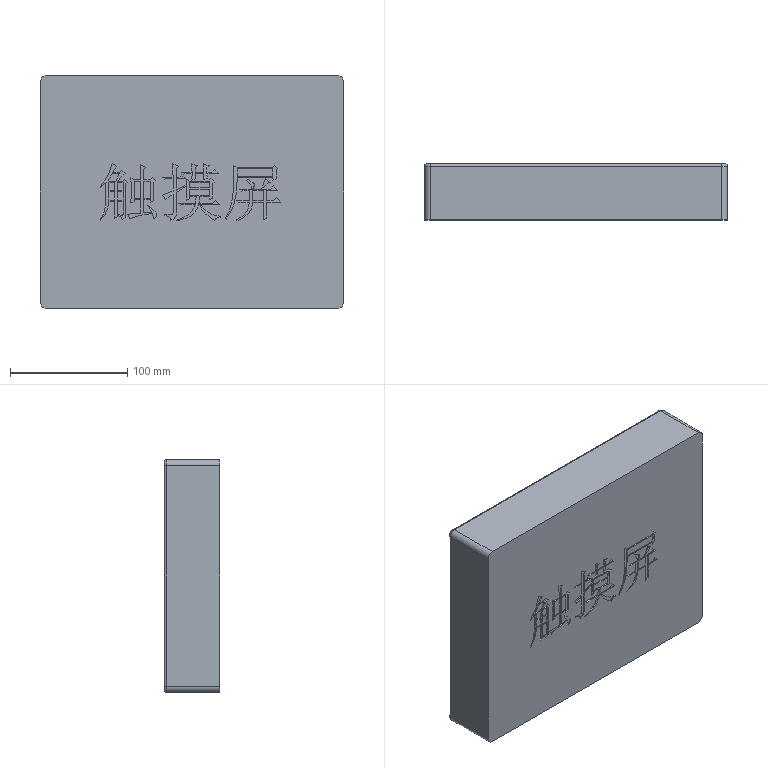Part | NX | 1 solid | 286 faces | box 258 x 47.5 x 198 mm | volume 2422965 mm3 | plane 199 | spline 70 | cylinder 13 | torus 4 | commonest cylinder face diameters 4 x4 10 x4 83.377 x1 146.201 x1 529.74 x1 561.552 x1